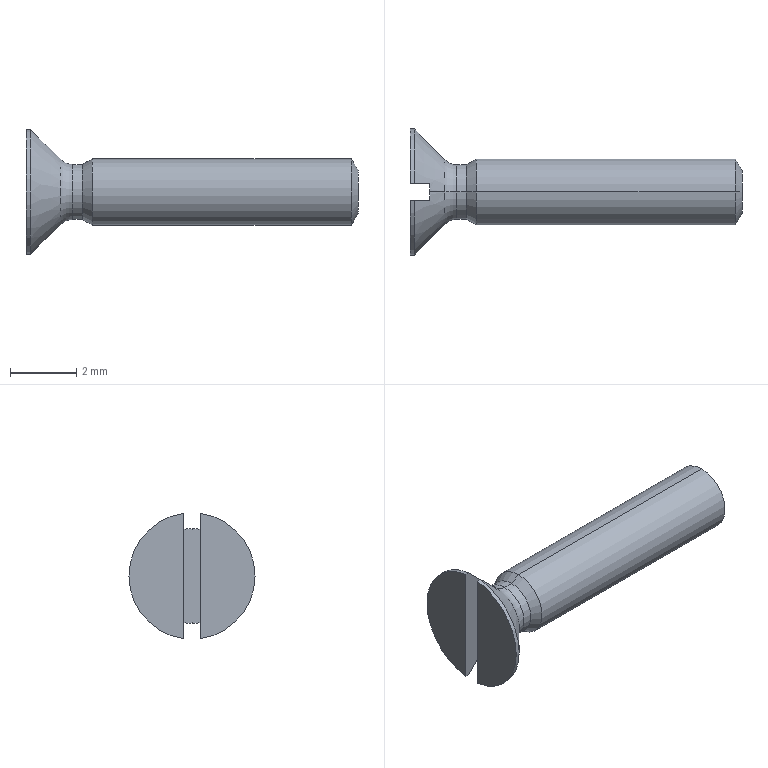Part | SolidWorks | features Chamfer 1, Cut 1, LPattern 1, RevCut 1, Revolution 1 | 1 solid | 20 faces | box 10 x 3.8 x 3.767 mm | volume 33.836 mm3 | cone 6 | cylinder 6 | plane 6 | torus 2 | commonest cylinder face diameters 1.654 x2 2 x2 3.8 x2
STEP:
#1=CARTESIAN_POINT('',(10.,0.,0.6536));
#2=VERTEX_POINT('',#1);
#3=CARTESIAN_POINT('',(10.,0.,-0.6536));
#4=VERTEX_POINT('',#3);
#5=CARTESIAN_POINT('',(10.,0.,0.));
#6=DIRECTION('',(-1.,0.,0.));
#7=DIRECTION('',(0.,0.,1.));
#8=AXIS2_PLACEMENT_3D('',#5,#6,#7);
#9=CIRCLE('',#8,0.6536);
#10=EDGE_CURVE('',#2,#4,#9,.T.);
#11=ORIENTED_EDGE('',*,*,#10,.T.);
#12=CARTESIAN_POINT('',(9.8,0.,-1.));
#13=VERTEX_POINT('',#12);
#14=CARTESIAN_POINT('',(9.8,0.,-1.));
#15=DIRECTION('',(-0.5,0.,-0.866));
#16=VECTOR('',#15,1000.);
#17=LINE('',#14,#16);
#18=EDGE_CURVE('',#4,#13,#17,.T.);
#19=ORIENTED_EDGE('',*,*,#18,.T.);
#20=CARTESIAN_POINT('',(9.8,0.,1.));
#21=VERTEX_POINT('',#20);
#22=CARTESIAN_POINT('',(9.8,0.,0.));
#23=DIRECTION('',(-1.,0.,0.));
#24=DIRECTION('',(0.,0.,1.));
#25=AXIS2_PLACEMENT_3D('',#22,#23,#24);
#26=CIRCLE('',#25,1.);
#27=EDGE_CURVE('',#21,#13,#26,.T.);
#28=ORIENTED_EDGE('',*,*,#27,.F.);
#29=CARTESIAN_POINT('',(9.8,0.,1.));
#30=DIRECTION('',(-0.5,0.,0.866));
#31=VECTOR('',#30,1000.);
#32=LINE('',#29,#31);
#33=EDGE_CURVE('',#2,#21,#32,.T.);
#34=ORIENTED_EDGE('',*,*,#33,.F.);
#35=EDGE_LOOP('',(#11,#19,#28,#34));
#36=FACE_OUTER_BOUND('',#35,.T.);
#37=CARTESIAN_POINT('',(9.8,0.,0.));
#38=DIRECTION('',(-1.,0.,0.));
#39=DIRECTION('',(0.,0.,1.));
#40=AXIS2_PLACEMENT_3D('',#37,#38,#39);
#41=CONICAL_SURFACE('',#40,1.,1.047);
#42=ADVANCED_FACE('',(#36),#41,.T.);
#43=ORIENTED_EDGE('',*,*,#27,.T.);
#44=CARTESIAN_POINT('',(2.,0.,-1.));
#45=VERTEX_POINT('',#44);
#46=CARTESIAN_POINT('',(0.,0.,-1.));
#47=DIRECTION('',(-1.,0.,0.));
#48=VECTOR('',#47,1000.);
#49=LINE('',#46,#48);
#50=EDGE_CURVE('',#13,#45,#49,.T.);
#51=ORIENTED_EDGE('',*,*,#50,.T.);
#52=CARTESIAN_POINT('',(2.,0.,1.));
#53=VERTEX_POINT('',#52);
#54=CARTESIAN_POINT('',(2.,0.,0.));
#55=DIRECTION('',(-1.,0.,0.));
#56=DIRECTION('',(0.,0.,1.));
#57=AXIS2_PLACEMENT_3D('',#54,#55,#56);
#58=CIRCLE('',#57,1.);
#59=EDGE_CURVE('',#53,#45,#58,.T.);
#60=ORIENTED_EDGE('',*,*,#59,.F.);
#61=CARTESIAN_POINT('',(0.,0.,1.));
#62=DIRECTION('',(-1.,0.,0.));
#63=VECTOR('',#62,1000.);
#64=LINE('',#61,#63);
#65=EDGE_CURVE('',#21,#53,#64,.T.);
#66=ORIENTED_EDGE('',*,*,#65,.F.);
#67=EDGE_LOOP('',(#43,#51,#60,#66));
#68=FACE_OUTER_BOUND('',#67,.T.);
#69=CARTESIAN_POINT('',(0.,0.,0.));
#70=DIRECTION('',(-1.,0.,0.));
#71=DIRECTION('',(0.,0.,1.));
#72=AXIS2_PLACEMENT_3D('',#69,#70,#71);
#73=CYLINDRICAL_SURFACE('',#72,1.);
#74=ADVANCED_FACE('',(#68),#73,.T.);
#75=CARTESIAN_POINT('',(1.7,0.,0.8268));
#76=VERTEX_POINT('',#75);
#77=CARTESIAN_POINT('',(1.7,0.,-0.8268));
#78=VERTEX_POINT('',#77);
#79=CARTESIAN_POINT('',(1.7,0.,0.));
#80=DIRECTION('',(-1.,0.,0.));
#81=DIRECTION('',(0.,0.,1.));
#82=AXIS2_PLACEMENT_3D('',#79,#80,#81);
#83=CIRCLE('',#82,0.8268);
#84=EDGE_CURVE('',#76,#78,#83,.T.);
#85=ORIENTED_EDGE('',*,*,#84,.F.);
#86=CARTESIAN_POINT('',(2.,0.,1.));
#87=DIRECTION('',(0.866,0.,0.5));
#88=VECTOR('',#87,1000.);
#89=LINE('',#86,#88);
#90=EDGE_CURVE('',#76,#53,#89,.T.);
#91=ORIENTED_EDGE('',*,*,#90,.T.);
#92=ORIENTED_EDGE('',*,*,#59,.T.);
#93=CARTESIAN_POINT('',(2.,0.,-1.));
#94=DIRECTION('',(0.866,0.,-0.5));
#95=VECTOR('',#94,1000.);
#96=LINE('',#93,#95);
#97=EDGE_CURVE('',#78,#45,#96,.T.);
#98=ORIENTED_EDGE('',*,*,#97,.F.);
#99=EDGE_LOOP('',(#85,#91,#92,#98));
#100=FACE_OUTER_BOUND('',#99,.T.);
#101=CARTESIAN_POINT('',(2.,0.,0.));
#102=DIRECTION('',(1.,0.,0.));
#103=DIRECTION('',(0.,0.,-1.));
#104=AXIS2_PLACEMENT_3D('',#101,#102,#103);
#105=CONICAL_SURFACE('',#104,1.,0.5236);
#106=ADVANCED_FACE('',(#100),#105,.T.);
#107=ORIENTED_EDGE('',*,*,#84,.T.);
#108=CARTESIAN_POINT('',(1.407,0.,-0.8268));
#109=VERTEX_POINT('',#108);
#110=CARTESIAN_POINT('',(0.,0.,-0.8268));
#111=DIRECTION('',(-1.,0.,0.));
#112=VECTOR('',#111,1000.);
#113=LINE('',#110,#112);
#114=EDGE_CURVE('',#78,#109,#113,.T.);
#115=ORIENTED_EDGE('',*,*,#114,.T.);
#116=CARTESIAN_POINT('',(1.407,0.,0.8268));
#117=VERTEX_POINT('',#116);
#118=CARTESIAN_POINT('',(1.407,0.,0.));
#119=DIRECTION('',(-1.,0.,0.));
#120=DIRECTION('',(0.,0.,1.));
#121=AXIS2_PLACEMENT_3D('',#118,#119,#120);
#122=CIRCLE('',#121,0.8268);
#123=EDGE_CURVE('',#117,#109,#122,.T.);
#124=ORIENTED_EDGE('',*,*,#123,.F.);
#125=CARTESIAN_POINT('',(0.,0.,0.8268));
#126=DIRECTION('',(-1.,0.,0.));
#127=VECTOR('',#126,1000.);
#128=LINE('',#125,#127);
#129=EDGE_CURVE('',#76,#117,#128,.T.);
#130=ORIENTED_EDGE('',*,*,#129,.F.);
#131=EDGE_LOOP('',(#107,#115,#124,#130));
#132=FACE_OUTER_BOUND('',#131,.T.);
#133=CARTESIAN_POINT('',(0.,0.,0.));
#134=DIRECTION('',(-1.,0.,0.));
#135=DIRECTION('',(0.,0.,1.));
#136=AXIS2_PLACEMENT_3D('',#133,#134,#135);
#137=CYLINDRICAL_SURFACE('',#136,0.8268);
#138=ADVANCED_FACE('',(#132),#137,.T.);
#139=CARTESIAN_POINT('',(1.054,0.,-0.9732));
#140=VERTEX_POINT('',#139);
#141=CARTESIAN_POINT('',(1.054,0.,0.9732));
#142=VERTEX_POINT('',#141);
#143=CARTESIAN_POINT('',(1.054,0.,0.));
#144=DIRECTION('',(-1.,0.,0.));
#145=DIRECTION('',(0.,0.,1.));
#146=AXIS2_PLACEMENT_3D('',#143,#144,#145);
#147=CIRCLE('',#146,0.9732);
#148=EDGE_CURVE('',#140,#142,#147,.T.);
#149=ORIENTED_EDGE('',*,*,#148,.F.);
#150=CARTESIAN_POINT('',(1.407,0.,-1.327));
#151=DIRECTION('',(0.,1.,0.));
#152=DIRECTION('',(0.,0.,1.));
#153=AXIS2_PLACEMENT_3D('',#150,#151,#152);
#154=CIRCLE('',#153,0.5);
#155=EDGE_CURVE('',#140,#109,#154,.T.);
#156=ORIENTED_EDGE('',*,*,#155,.T.);
#157=CARTESIAN_POINT('',(1.407,0.,0.));
#158=DIRECTION('',(-1.,0.,0.));
#159=DIRECTION('',(0.,0.,1.));
#160=AXIS2_PLACEMENT_3D('',#157,#158,#159);
#161=CIRCLE('',#160,0.8268);
#162=EDGE_CURVE('',#109,#117,#161,.T.);
#163=ORIENTED_EDGE('',*,*,#162,.T.);
#164=CARTESIAN_POINT('',(1.407,0.,1.327));
#165=DIRECTION('',(0.,-1.,0.));
#166=DIRECTION('',(0.,0.,-1.));
#167=AXIS2_PLACEMENT_3D('',#164,#165,#166);
#168=CIRCLE('',#167,0.5);
#169=EDGE_CURVE('',#142,#117,#168,.T.);
#170=ORIENTED_EDGE('',*,*,#169,.F.);
#171=EDGE_LOOP('',(#149,#156,#163,#170));
#172=FACE_OUTER_BOUND('',#171,.T.);
#173=CARTESIAN_POINT('',(1.407,0.,0.));
#174=DIRECTION('',(-1.,0.,0.));
#175=DIRECTION('',(0.,0.,1.));
#176=AXIS2_PLACEMENT_3D('',#173,#174,#175);
#177=TOROIDAL_SURFACE('',#176,1.327,0.5);
#178=ADVANCED_FACE('',(#172),#177,.F.);
#179=CARTESIAN_POINT('',(1.054,0.,0.));
#180=DIRECTION('',(-1.,0.,0.));
#181=DIRECTION('',(0.,0.,1.));
#182=AXIS2_PLACEMENT_3D('',#179,#180,#181);
#183=CIRCLE('',#182,0.9732);
#184=EDGE_CURVE('',#142,#140,#183,.T.);
#185=ORIENTED_EDGE('',*,*,#184,.T.);
#186=CARTESIAN_POINT('',(0.6,0.,-1.427));
#187=VERTEX_POINT('',#186);
#188=CARTESIAN_POINT('',(1.054,0.,-0.9732));
#189=DIRECTION('',(-0.7071,0.,-0.7071));
#190=VECTOR('',#189,1000.);
#191=LINE('',#188,#190);
#192=EDGE_CURVE('',#140,#187,#191,.T.);
#193=ORIENTED_EDGE('',*,*,#192,.T.);
#194=CARTESIAN_POINT('',(0.6,0.25,-1.405));
#195=VERTEX_POINT('',#194);
#196=CARTESIAN_POINT('',(0.6,0.,0.));
#197=DIRECTION('',(-1.,0.,0.));
#198=DIRECTION('',(0.,0.,1.));
#199=AXIS2_PLACEMENT_3D('',#196,#197,#198);
#200=CIRCLE('',#199,1.427);
#201=EDGE_CURVE('',#195,#187,#200,.T.);
#202=ORIENTED_EDGE('',*,*,#201,.F.);
#203=CARTESIAN_POINT('',(0.1268,0.25,-1.883));
#204=VERTEX_POINT('',#203);
#205=CARTESIAN_POINT('',(0.6,0.25,-1.405));
#206=CARTESIAN_POINT('',(0.4426,0.25,-1.565));
#207=CARTESIAN_POINT('',(0.2848,0.25,-1.724));
#208=CARTESIAN_POINT('',(0.1268,0.25,-1.883));
#209=B_SPLINE_CURVE_WITH_KNOTS('',3,(#205,#206,#207,#208),.UNSPECIFIED.,.F.,.F.,(4,4),(0.007598,0.008274),.UNSPECIFIED.);
#210=EDGE_CURVE('',#195,#204,#209,.T.);
#211=ORIENTED_EDGE('',*,*,#210,.T.);
#212=CARTESIAN_POINT('',(0.1268,0.25,1.883));
#213=VERTEX_POINT('',#212);
#214=CARTESIAN_POINT('',(0.1268,0.,0.));
#215=DIRECTION('',(-1.,0.,0.));
#216=DIRECTION('',(0.,0.,1.));
#217=AXIS2_PLACEMENT_3D('',#214,#215,#216);
#218=CIRCLE('',#217,1.9);
#219=EDGE_CURVE('',#213,#204,#218,.T.);
#220=ORIENTED_EDGE('',*,*,#219,.F.);
#221=CARTESIAN_POINT('',(0.6,0.25,1.405));
#222=VERTEX_POINT('',#221);
#223=CARTESIAN_POINT('',(0.1268,0.25,1.883));
#224=CARTESIAN_POINT('',(0.2848,0.25,1.724));
#225=CARTESIAN_POINT('',(0.4426,0.25,1.565));
#226=CARTESIAN_POINT('',(0.6,0.25,1.405));
#227=B_SPLINE_CURVE_WITH_KNOTS('',3,(#223,#224,#225,#226),.UNSPECIFIED.,.F.,.F.,(4,4),(0.003215,0.003889),.UNSPECIFIED.);
#228=EDGE_CURVE('',#213,#222,#227,.T.);
#229=ORIENTED_EDGE('',*,*,#228,.T.);
#230=CARTESIAN_POINT('',(0.6,0.,1.427));
#231=VERTEX_POINT('',#230);
#232=CARTESIAN_POINT('',(0.6,0.,0.));
#233=DIRECTION('',(-1.,0.,0.));
#234=DIRECTION('',(0.,0.,1.));
#235=AXIS2_PLACEMENT_3D('',#232,#233,#234);
#236=CIRCLE('',#235,1.427);
#237=EDGE_CURVE('',#231,#222,#236,.T.);
#238=ORIENTED_EDGE('',*,*,#237,.F.);
#239=CARTESIAN_POINT('',(1.054,0.,0.9732));
#240=DIRECTION('',(-0.7071,0.,0.7071));
#241=VECTOR('',#240,1000.);
#242=LINE('',#239,#241);
#243=EDGE_CURVE('',#142,#231,#242,.T.);
#244=ORIENTED_EDGE('',*,*,#243,.F.);
#245=EDGE_LOOP('',(#185,#193,#202,#211,#220,#229,#238,#244));
#246=FACE_OUTER_BOUND('',#245,.T.);
#247=CARTESIAN_POINT('',(1.054,0.,0.));
#248=DIRECTION('',(-1.,0.,0.));
#249=DIRECTION('',(0.,0.,1.));
#250=AXIS2_PLACEMENT_3D('',#247,#248,#249);
#251=CONICAL_SURFACE('',#250,0.9732,0.7854);
#252=ADVANCED_FACE('',(#246),#251,.T.);
#253=CARTESIAN_POINT('',(0.,0.25,1.883));
#254=VERTEX_POINT('',#253);
#255=CARTESIAN_POINT('',(0.,0.25,-1.883));
#256=VERTEX_POINT('',#255);
#257=CARTESIAN_POINT('',(0.,0.,0.));
#258=DIRECTION('',(-1.,0.,0.));
#259=DIRECTION('',(0.,0.,1.));
#260=AXIS2_PLACEMENT_3D('',#257,#258,#259);
#261=CIRCLE('',#260,1.9);
#262=EDGE_CURVE('',#254,#256,#261,.T.);
#263=ORIENTED_EDGE('',*,*,#262,.T.);
#264=CARTESIAN_POINT('',(0.,0.25,-1.883));
#265=DIRECTION('',(0.,0.,-1.));
#266=VECTOR('',#265,1000.);
#267=LINE('',#264,#266);
#268=EDGE_CURVE('',#254,#256,#267,.T.);
#269=ORIENTED_EDGE('',*,*,#268,.F.);
#270=EDGE_LOOP('',(#263,#269));
#271=FACE_OUTER_BOUND('',#270,.T.);
#272=CARTESIAN_POINT('',(0.,0.,0.));
#273=DIRECTION('',(1.,0.,0.));
#274=DIRECTION('',(0.,0.,-1.));
#275=AXIS2_PLACEMENT_3D('',#272,#273,#274);
#276=PLANE('',#275);
#277=ADVANCED_FACE('',(#271),#276,.F.);
#278=ORIENTED_EDGE('',*,*,#219,.T.);
#279=CARTESIAN_POINT('',(0.6,0.25,-1.883));
#280=DIRECTION('',(-1.,0.,0.));
#281=VECTOR('',#280,1000.);
#282=LINE('',#279,#281);
#283=EDGE_CURVE('',#204,#256,#282,.T.);
#284=ORIENTED_EDGE('',*,*,#283,.T.);
#285=ORIENTED_EDGE('',*,*,#262,.F.);
#286=CARTESIAN_POINT('',(0.6,0.25,1.883));
#287=DIRECTION('',(-1.,0.,0.));
#288=VECTOR('',#287,1000.);
#289=LINE('',#286,#288);
#290=EDGE_CURVE('',#213,#254,#289,.T.);
#291=ORIENTED_EDGE('',*,*,#290,.F.);
#292=EDGE_LOOP('',(#278,#284,#285,#291));
#293=FACE_OUTER_BOUND('',#292,.T.);
#294=CARTESIAN_POINT('',(0.,0.,0.));
#295=DIRECTION('',(-1.,0.,0.));
#296=DIRECTION('',(0.,0.,1.));
#297=AXIS2_PLACEMENT_3D('',#294,#295,#296);
#298=CYLINDRICAL_SURFACE('',#297,1.9);
#299=ADVANCED_FACE('',(#293),#298,.T.);
#300=CARTESIAN_POINT('',(0.,-0.25,-1.883));
#301=VERTEX_POINT('',#300);
#302=CARTESIAN_POINT('',(0.,-0.25,1.883));
#303=VERTEX_POINT('',#302);
#304=CARTESIAN_POINT('',(0.,0.,0.));
#305=DIRECTION('',(-1.,0.,0.));
#306=DIRECTION('',(0.,0.,1.));
#307=AXIS2_PLACEMENT_3D('',#304,#305,#306);
#308=CIRCLE('',#307,1.9);
#309=EDGE_CURVE('',#301,#303,#308,.T.);
#310=ORIENTED_EDGE('',*,*,#309,.T.);
#311=CARTESIAN_POINT('',(0.,-0.25,-1.883));
#312=DIRECTION('',(0.,0.,1.));
#313=VECTOR('',#312,1000.);
#314=LINE('',#311,#313);
#315=EDGE_CURVE('',#301,#303,#314,.T.);
#316=ORIENTED_EDGE('',*,*,#315,.F.);
#317=EDGE_LOOP('',(#310,#316));
#318=FACE_OUTER_BOUND('',#317,.T.);
#319=CARTESIAN_POINT('',(0.,0.,0.));
#320=DIRECTION('',(1.,0.,0.));
#321=DIRECTION('',(0.,0.,-1.));
#322=AXIS2_PLACEMENT_3D('',#319,#320,#321);
#323=PLANE('',#322);
#324=ADVANCED_FACE('',(#318),#323,.F.);
#325=CARTESIAN_POINT('',(0.1268,-0.25,-1.883));
#326=VERTEX_POINT('',#325);
#327=CARTESIAN_POINT('',(0.1268,-0.25,1.883));
#328=VERTEX_POINT('',#327);
#329=CARTESIAN_POINT('',(0.1268,0.,0.));
#330=DIRECTION('',(-1.,0.,0.));
#331=DIRECTION('',(0.,0.,1.));
#332=AXIS2_PLACEMENT_3D('',#329,#330,#331);
#333=CIRCLE('',#332,1.9);
#334=EDGE_CURVE('',#326,#328,#333,.T.);
#335=ORIENTED_EDGE('',*,*,#334,.T.);
#336=CARTESIAN_POINT('',(0.6,-0.25,1.883));
#337=DIRECTION('',(-1.,0.,0.));
#338=VECTOR('',#337,1000.);
#339=LINE('',#336,#338);
#340=EDGE_CURVE('',#328,#303,#339,.T.);
#341=ORIENTED_EDGE('',*,*,#340,.T.);
#342=ORIENTED_EDGE('',*,*,#309,.F.);
#343=CARTESIAN_POINT('',(0.6,-0.25,-1.883));
#344=DIRECTION('',(-1.,0.,0.));
#345=VECTOR('',#344,1000.);
#346=LINE('',#343,#345);
#347=EDGE_CURVE('',#326,#301,#346,.T.);
#348=ORIENTED_EDGE('',*,*,#347,.F.);
#349=EDGE_LOOP('',(#335,#341,#342,#348));
#350=FACE_OUTER_BOUND('',#349,.T.);
#351=CARTESIAN_POINT('',(0.,0.,0.));
#352=DIRECTION('',(-1.,0.,0.));
#353=DIRECTION('',(0.,0.,1.));
#354=AXIS2_PLACEMENT_3D('',#351,#352,#353);
#355=CYLINDRICAL_SURFACE('',#354,1.9);
#356=ADVANCED_FACE('',(#350),#355,.T.);
#357=ORIENTED_EDGE('',*,*,#192,.F.);
#358=ORIENTED_EDGE('',*,*,#148,.T.);
#359=ORIENTED_EDGE('',*,*,#243,.T.);
#360=CARTESIAN_POINT('',(0.6,-0.25,1.405));
#361=VERTEX_POINT('',#360);
#362=CARTESIAN_POINT('',(0.6,0.,0.));
#363=DIRECTION('',(-1.,0.,0.));
#364=DIRECTION('',(0.,0.,1.));
#365=AXIS2_PLACEMENT_3D('',#362,#363,#364);
#366=CIRCLE('',#365,1.427);
#367=EDGE_CURVE('',#361,#231,#366,.T.);
#368=ORIENTED_EDGE('',*,*,#367,.F.);
#369=CARTESIAN_POINT('',(0.6,-0.25,1.405));
#370=CARTESIAN_POINT('',(0.4426,-0.25,1.565));
#371=CARTESIAN_POINT('',(0.2848,-0.25,1.724));
#372=CARTESIAN_POINT('',(0.1268,-0.25,1.883));
#373=B_SPLINE_CURVE_WITH_KNOTS('',3,(#369,#370,#371,#372),.UNSPECIFIED.,.F.,.F.,(4,4),(0.007598,0.008274),.UNSPECIFIED.);
#374=EDGE_CURVE('',#361,#328,#373,.T.);
#375=ORIENTED_EDGE('',*,*,#374,.T.);
#376=ORIENTED_EDGE('',*,*,#334,.F.);
#377=CARTESIAN_POINT('',(0.6,-0.25,-1.405));
#378=VERTEX_POINT('',#377);
#379=CARTESIAN_POINT('',(0.1268,-0.25,-1.883));
#380=CARTESIAN_POINT('',(0.2848,-0.25,-1.724));
#381=CARTESIAN_POINT('',(0.4426,-0.25,-1.565));
#382=CARTESIAN_POINT('',(0.6,-0.25,-1.405));
#383=B_SPLINE_CURVE_WITH_KNOTS('',3,(#379,#380,#381,#382),.UNSPECIFIED.,.F.,.F.,(4,4),(0.003215,0.003889),.UNSPECIFIED.);
#384=EDGE_CURVE('',#326,#378,#383,.T.);
#385=ORIENTED_EDGE('',*,*,#384,.T.);
#386=CARTESIAN_POINT('',(0.6,0.,0.));
#387=DIRECTION('',(-1.,0.,0.));
#388=DIRECTION('',(0.,0.,1.));
#389=AXIS2_PLACEMENT_3D('',#386,#387,#388);
#390=CIRCLE('',#389,1.427);
#391=EDGE_CURVE('',#187,#378,#390,.T.);
#392=ORIENTED_EDGE('',*,*,#391,.F.);
#393=EDGE_LOOP('',(#357,#358,#359,#368,#375,#376,#385,#392));
#394=FACE_OUTER_BOUND('',#393,.T.);
#395=CARTESIAN_POINT('',(1.054,0.,0.));
#396=DIRECTION('',(-1.,0.,0.));
#397=DIRECTION('',(0.,0.,1.));
#398=AXIS2_PLACEMENT_3D('',#395,#396,#397);
#399=CONICAL_SURFACE('',#398,0.9732,0.7854);
#400=ADVANCED_FACE('',(#394),#399,.T.);
#401=ORIENTED_EDGE('',*,*,#155,.F.);
#402=ORIENTED_EDGE('',*,*,#184,.F.);
#403=ORIENTED_EDGE('',*,*,#169,.T.);
#404=ORIENTED_EDGE('',*,*,#123,.T.);
#405=EDGE_LOOP('',(#401,#402,#403,#404));
#406=FACE_OUTER_BOUND('',#405,.T.);
#407=CARTESIAN_POINT('',(1.407,0.,0.));
#408=DIRECTION('',(-1.,0.,0.));
#409=DIRECTION('',(0.,0.,1.));
#410=AXIS2_PLACEMENT_3D('',#407,#408,#409);
#411=TOROIDAL_SURFACE('',#410,1.327,0.5);
#412=ADVANCED_FACE('',(#406),#411,.F.);
#413=ORIENTED_EDGE('',*,*,#114,.F.);
#414=CARTESIAN_POINT('',(1.7,0.,0.));
#415=DIRECTION('',(-1.,0.,0.));
#416=DIRECTION('',(0.,0.,1.));
#417=AXIS2_PLACEMENT_3D('',#414,#415,#416);
#418=CIRCLE('',#417,0.8268);
#419=EDGE_CURVE('',#78,#76,#418,.T.);
#420=ORIENTED_EDGE('',*,*,#419,.T.);
#421=ORIENTED_EDGE('',*,*,#129,.T.);
#422=ORIENTED_EDGE('',*,*,#162,.F.);
#423=EDGE_LOOP('',(#413,#420,#421,#422));
#424=FACE_OUTER_BOUND('',#423,.T.);
#425=CARTESIAN_POINT('',(0.,0.,0.));
#426=DIRECTION('',(-1.,0.,0.));
#427=DIRECTION('',(0.,0.,1.));
#428=AXIS2_PLACEMENT_3D('',#425,#426,#427);
#429=CYLINDRICAL_SURFACE('',#428,0.8268);
#430=ADVANCED_FACE('',(#424),#429,.T.);
#431=ORIENTED_EDGE('',*,*,#90,.F.);
#432=ORIENTED_EDGE('',*,*,#419,.F.);
#433=ORIENTED_EDGE('',*,*,#97,.T.);
#434=CARTESIAN_POINT('',(2.,0.,0.));
#435=DIRECTION('',(-1.,0.,0.));
#436=DIRECTION('',(0.,0.,1.));
#437=AXIS2_PLACEMENT_3D('',#434,#435,#436);
#438=CIRCLE('',#437,1.);
#439=EDGE_CURVE('',#45,#53,#438,.T.);
#440=ORIENTED_EDGE('',*,*,#439,.T.);
#441=EDGE_LOOP('',(#431,#432,#433,#440));
#442=FACE_OUTER_BOUND('',#441,.T.);
#443=CARTESIAN_POINT('',(2.,0.,0.));
#444=DIRECTION('',(1.,0.,0.));
#445=DIRECTION('',(0.,0.,-1.));
#446=AXIS2_PLACEMENT_3D('',#443,#444,#445);
#447=CONICAL_SURFACE('',#446,1.,0.5236);
#448=ADVANCED_FACE('',(#442),#447,.T.);
#449=ORIENTED_EDGE('',*,*,#50,.F.);
#450=CARTESIAN_POINT('',(9.8,0.,0.));
#451=DIRECTION('',(-1.,0.,0.));
#452=DIRECTION('',(0.,0.,1.));
#453=AXIS2_PLACEMENT_3D('',#450,#451,#452);
#454=CIRCLE('',#453,1.);
#455=EDGE_CURVE('',#13,#21,#454,.T.);
#456=ORIENTED_EDGE('',*,*,#455,.T.);
#457=ORIENTED_EDGE('',*,*,#65,.T.);
#458=ORIENTED_EDGE('',*,*,#439,.F.);
#459=EDGE_LOOP('',(#449,#456,#457,#458));
#460=FACE_OUTER_BOUND('',#459,.T.);
#461=CARTESIAN_POINT('',(0.,0.,0.));
#462=DIRECTION('',(-1.,0.,0.));
#463=DIRECTION('',(0.,0.,1.));
#464=AXIS2_PLACEMENT_3D('',#461,#462,#463);
#465=CYLINDRICAL_SURFACE('',#464,1.);
#466=ADVANCED_FACE('',(#460),#465,.T.);
#467=ORIENTED_EDGE('',*,*,#290,.T.);
#468=ORIENTED_EDGE('',*,*,#268,.T.);
#469=ORIENTED_EDGE('',*,*,#283,.F.);
#470=ORIENTED_EDGE('',*,*,#210,.F.);
#471=CARTESIAN_POINT('',(0.6,0.25,-1.883));
#472=DIRECTION('',(0.,0.,-1.));
#473=VECTOR('',#472,1000.);
#474=LINE('',#471,#473);
#475=EDGE_CURVE('',#222,#195,#474,.T.);
#476=ORIENTED_EDGE('',*,*,#475,.F.);
#477=ORIENTED_EDGE('',*,*,#228,.F.);
#478=EDGE_LOOP('',(#467,#468,#469,#470,#476,#477));
#479=FACE_OUTER_BOUND('',#478,.T.);
#480=CARTESIAN_POINT('',(0.6,0.25,-1.883));
#481=DIRECTION('',(0.,1.,0.));
#482=DIRECTION('',(0.,0.,1.));
#483=AXIS2_PLACEMENT_3D('',#480,#481,#482);
#484=PLANE('',#483);
#485=ADVANCED_FACE('',(#479),#484,.F.);
#486=ORIENTED_EDGE('',*,*,#347,.T.);
#487=ORIENTED_EDGE('',*,*,#315,.T.);
#488=ORIENTED_EDGE('',*,*,#340,.F.);
#489=ORIENTED_EDGE('',*,*,#374,.F.);
#490=CARTESIAN_POINT('',(0.6,-0.25,-1.883));
#491=DIRECTION('',(0.,0.,1.));
#492=VECTOR('',#491,1000.);
#493=LINE('',#490,#492);
#494=EDGE_CURVE('',#378,#361,#493,.T.);
#495=ORIENTED_EDGE('',*,*,#494,.F.);
#496=ORIENTED_EDGE('',*,*,#384,.F.);
#497=EDGE_LOOP('',(#486,#487,#488,#489,#495,#496));
#498=FACE_OUTER_BOUND('',#497,.T.);
#499=CARTESIAN_POINT('',(0.6,-0.25,-1.883));
#500=DIRECTION('',(0.,-1.,0.));
#501=DIRECTION('',(0.,0.,-1.));
#502=AXIS2_PLACEMENT_3D('',#499,#500,#501);
#503=PLANE('',#502);
#504=ADVANCED_FACE('',(#498),#503,.F.);
#505=ORIENTED_EDGE('',*,*,#201,.T.);
#506=ORIENTED_EDGE('',*,*,#391,.T.);
#507=ORIENTED_EDGE('',*,*,#494,.T.);
#508=ORIENTED_EDGE('',*,*,#367,.T.);
#509=ORIENTED_EDGE('',*,*,#237,.T.);
#510=ORIENTED_EDGE('',*,*,#475,.T.);
#511=EDGE_LOOP('',(#505,#506,#507,#508,#509,#510));
#512=FACE_OUTER_BOUND('',#511,.T.);
#513=CARTESIAN_POINT('',(0.6,0.,0.));
#514=DIRECTION('',(-1.,0.,0.));
#515=DIRECTION('',(0.,0.,1.));
#516=AXIS2_PLACEMENT_3D('',#513,#514,#515);
#517=PLANE('',#516);
#518=ADVANCED_FACE('',(#512),#517,.T.);
#519=ORIENTED_EDGE('',*,*,#18,.F.);
#520=CARTESIAN_POINT('',(10.,0.,0.));
#521=DIRECTION('',(-1.,0.,0.));
#522=DIRECTION('',(0.,0.,1.));
#523=AXIS2_PLACEMENT_3D('',#520,#521,#522);
#524=CIRCLE('',#523,0.6536);
#525=EDGE_CURVE('',#4,#2,#524,.T.);
#526=ORIENTED_EDGE('',*,*,#525,.T.);
#527=ORIENTED_EDGE('',*,*,#33,.T.);
#528=ORIENTED_EDGE('',*,*,#455,.F.);
#529=EDGE_LOOP('',(#519,#526,#527,#528));
#530=FACE_OUTER_BOUND('',#529,.T.);
#531=CARTESIAN_POINT('',(9.8,0.,0.));
#532=DIRECTION('',(-1.,0.,0.));
#533=DIRECTION('',(0.,0.,1.));
#534=AXIS2_PLACEMENT_3D('',#531,#532,#533);
#535=CONICAL_SURFACE('',#534,1.,1.047);
#536=ADVANCED_FACE('',(#530),#535,.T.);
#537=ORIENTED_EDGE('',*,*,#10,.F.);
#538=ORIENTED_EDGE('',*,*,#525,.F.);
#539=EDGE_LOOP('',(#537,#538));
#540=FACE_OUTER_BOUND('',#539,.T.);
#541=CARTESIAN_POINT('',(10.,1.,0.));
#542=DIRECTION('',(-1.,0.,0.));
#543=DIRECTION('',(0.,0.,1.));
#544=AXIS2_PLACEMENT_3D('',#541,#542,#543);
#545=PLANE('',#544);
#546=ADVANCED_FACE('',(#540),#545,.F.);
#547=CLOSED_SHELL('',(#42,#74,#106,#138,#178,#252,#277,#299,#324,#356,#400,#412,#430,#448,#466,#485,#504,#518,#536,#546));
#548=MANIFOLD_SOLID_BREP('',#547);
#549=CARTESIAN_POINT('',(0.,0.,0.));
#550=DIRECTION('',(0.,0.,1.));
#551=DIRECTION('',(1.,0.,0.));
#552=AXIS2_PLACEMENT_3D('',#549,#550,#551);
#553=(LENGTH_UNIT()NAMED_UNIT(*)SI_UNIT(.MILLI.,.METRE.));
#554=UNCERTAINTY_MEASURE_WITH_UNIT(LENGTH_MEASURE(0.00001),#553,'','');
#555=(NAMED_UNIT(*)PLANE_ANGLE_UNIT()SI_UNIT($,.RADIAN.));
#556=(NAMED_UNIT(*)SI_UNIT($,.STERADIAN.)SOLID_ANGLE_UNIT());
#557=(GEOMETRIC_REPRESENTATION_CONTEXT(3)GLOBAL_UNCERTAINTY_ASSIGNED_CONTEXT((#554))GLOBAL_UNIT_ASSIGNED_CONTEXT((#553,#555,#556))REPRESENTATION_CONTEXT('',''));
#558=ADVANCED_BREP_SHAPE_REPRESENTATION('',(#548,#552),#557);